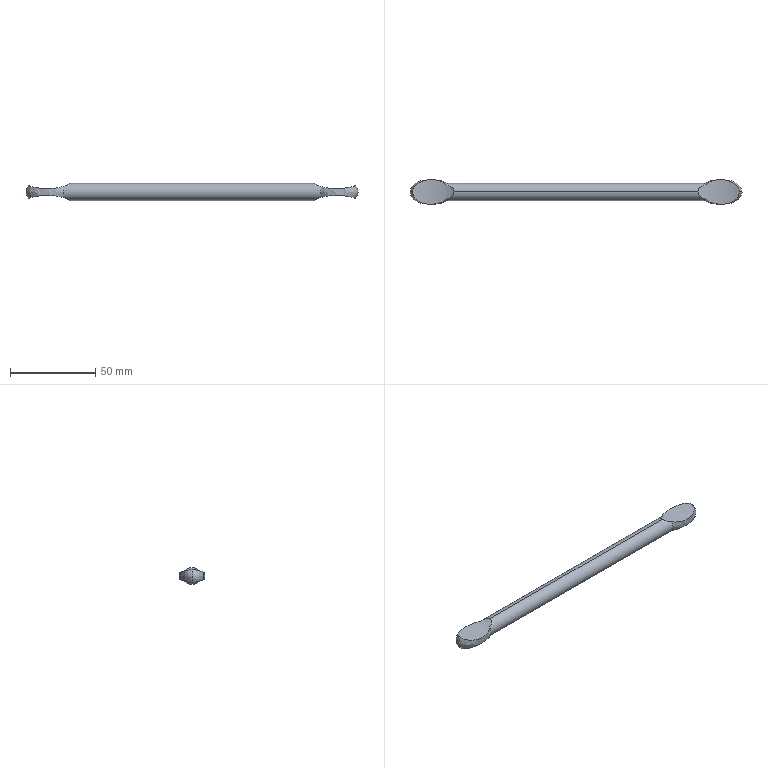Part | SolidWorks | features Extrusion 1, ICE 1, MirrorPattern 1, Revolution 1 | 1 solid | 10 faces | box 195 x 14.893 x 10 mm | volume 14339 mm3 | spline 8 | cylinder 2 | commonest cylinder face diameters 10 x2
STEP:
#1=CARTESIAN_POINT('',(97.5,0.,0.));
#2=VERTEX_POINT('',#1);
#3=CARTESIAN_POINT('',(95.865,0.,-3.708));
#4=VERTEX_POINT('',#3);
#5=CARTESIAN_POINT('',(97.5,0.,0.));
#6=CARTESIAN_POINT('',(97.5,0.,-1.308));
#7=CARTESIAN_POINT('',(96.943,0.,-2.572));
#8=CARTESIAN_POINT('',(95.865,0.,-3.708));
#9=(BOUNDED_CURVE()B_SPLINE_CURVE(3,(#5,#6,#7,#8),.UNSPECIFIED.,.F.,.T.)B_SPLINE_CURVE_WITH_KNOTS((4,4),(0.,0.5172),.UNSPECIFIED.)CURVE()GEOMETRIC_REPRESENTATION_ITEM()RATIONAL_B_SPLINE_CURVE((1.,0.9778,0.9778,1.))REPRESENTATION_ITEM(''));
#10=EDGE_CURVE('',#2,#4,#9,.T.);
#11=ORIENTED_EDGE('',*,*,#10,.F.);
#12=CARTESIAN_POINT('',(95.865,0.,3.708));
#13=VERTEX_POINT('',#12);
#14=CARTESIAN_POINT('',(97.5,0.,0.));
#15=CARTESIAN_POINT('',(97.5,0.,1.308));
#16=CARTESIAN_POINT('',(96.943,0.,2.572));
#17=CARTESIAN_POINT('',(95.865,0.,3.708));
#18=(BOUNDED_CURVE()B_SPLINE_CURVE(3,(#14,#15,#16,#17),.UNSPECIFIED.,.F.,.T.)B_SPLINE_CURVE_WITH_KNOTS((4,4),(0.,0.5172),.UNSPECIFIED.)CURVE()GEOMETRIC_REPRESENTATION_ITEM()RATIONAL_B_SPLINE_CURVE((1.,0.9778,0.9778,1.))REPRESENTATION_ITEM(''));
#19=EDGE_CURVE('',#2,#13,#18,.T.);
#20=ORIENTED_EDGE('',*,*,#19,.T.);
#21=CARTESIAN_POINT('',(75.683,-3.851,3.19));
#22=VERTEX_POINT('',#21);
#23=CARTESIAN_POINT('',(95.865,0.,3.708));
#24=CARTESIAN_POINT('',(95.865,-0.2608,3.708));
#25=CARTESIAN_POINT('',(95.846,-0.5214,3.701));
#26=CARTESIAN_POINT('',(95.771,-1.032,3.672));
#27=CARTESIAN_POINT('',(95.716,-1.283,3.651));
#28=CARTESIAN_POINT('',(95.569,-1.778,3.597));
#29=CARTESIAN_POINT('',(95.477,-2.023,3.564));
#30=CARTESIAN_POINT('',(95.265,-2.49,3.489));
#31=CARTESIAN_POINT('',(95.144,-2.715,3.448));
#32=CARTESIAN_POINT('',(94.875,-3.149,3.359));
#33=CARTESIAN_POINT('',(94.725,-3.359,3.312));
#34=CARTESIAN_POINT('',(94.406,-3.757,3.215));
#35=CARTESIAN_POINT('',(94.236,-3.945,3.166));
#36=CARTESIAN_POINT('',(93.701,-4.481,3.017));
#37=CARTESIAN_POINT('',(93.306,-4.803,2.917));
#38=CARTESIAN_POINT('',(92.462,-5.379,2.725));
#39=CARTESIAN_POINT('',(92.021,-5.629,2.636));
#40=CARTESIAN_POINT('',(91.107,-6.069,2.473));
#41=CARTESIAN_POINT('',(90.635,-6.259,2.399));
#42=CARTESIAN_POINT('',(89.662,-6.587,2.269));
#43=CARTESIAN_POINT('',(89.163,-6.725,2.213));
#44=CARTESIAN_POINT('',(88.157,-6.948,2.12));
#45=CARTESIAN_POINT('',(87.647,-7.035,2.083));
#46=CARTESIAN_POINT('',(86.619,-7.162,2.029));
#47=CARTESIAN_POINT('',(86.103,-7.202,2.012));
#48=CARTESIAN_POINT('',(85.068,-7.236,1.997));
#49=CARTESIAN_POINT('',(84.548,-7.23,1.999));
#50=CARTESIAN_POINT('',(82.998,-7.145,2.036));
#51=CARTESIAN_POINT('',(81.968,-6.997,2.1));
#52=CARTESIAN_POINT('',(80.468,-6.625,2.254));
#53=CARTESIAN_POINT('',(79.973,-6.474,2.315));
#54=CARTESIAN_POINT('',(79.014,-6.12,2.453));
#55=CARTESIAN_POINT('',(78.55,-5.916,2.531));
#56=CARTESIAN_POINT('',(77.656,-5.448,2.701));
#57=CARTESIAN_POINT('',(77.227,-5.183,2.793));
#58=CARTESIAN_POINT('',(76.614,-4.726,2.939));
#59=CARTESIAN_POINT('',(76.415,-4.564,2.989));
#60=CARTESIAN_POINT('',(76.035,-4.221,3.089));
#61=CARTESIAN_POINT('',(75.854,-4.041,3.14));
#62=CARTESIAN_POINT('',(75.683,-3.851,3.19));
#63=B_SPLINE_CURVE_WITH_KNOTS('',3,(#23,#24,#25,#26,#27,#28,#29,#30,#31,#32,#33,#34,#35,#36,#37,#38,#39,#40,#41,#42,#43,#44,#45,#46,#47,#48,#49,#50,#51,#52,#53,#54,#55,#56,#57,#58,#59,#60,#61,#62),.UNSPECIFIED.,.F.,.F.,(4,2,2,2,2,2,2,2,2,2,2,2,2,2,2,2,2,2,2,4),(0.02466,0.02543,0.0262,0.02697,0.02773,0.0285,0.02927,0.03081,0.03235,0.03389,0.03542,0.03696,0.0385,0.04004,0.04311,0.04465,0.04619,0.04773,0.04849,0.04926),.UNSPECIFIED.);
#64=EDGE_CURVE('',#13,#22,#63,.T.);
#65=ORIENTED_EDGE('',*,*,#64,.T.);
#66=CARTESIAN_POINT('',(75.683,-3.851,-3.19));
#67=VERTEX_POINT('',#66);
#68=CARTESIAN_POINT('',(75.683,0.,0.));
#69=DIRECTION('',(1.,0.,0.));
#70=DIRECTION('',(0.,0.,1.));
#71=AXIS2_PLACEMENT_3D('',#68,#69,#70);
#72=CIRCLE('',#71,5.);
#73=EDGE_CURVE('',#22,#67,#72,.T.);
#74=ORIENTED_EDGE('',*,*,#73,.T.);
#75=CARTESIAN_POINT('',(75.683,-3.851,-3.19));
#76=CARTESIAN_POINT('',(76.026,-4.232,-3.09));
#77=CARTESIAN_POINT('',(76.404,-4.569,-2.989));
#78=CARTESIAN_POINT('',(77.218,-5.177,-2.795));
#79=CARTESIAN_POINT('',(77.657,-5.448,-2.7));
#80=CARTESIAN_POINT('',(79.01,-6.157,-2.444));
#81=CARTESIAN_POINT('',(79.969,-6.501,-2.305));
#82=CARTESIAN_POINT('',(81.473,-6.874,-2.151));
#83=CARTESIAN_POINT('',(81.981,-6.973,-2.109));
#84=CARTESIAN_POINT('',(83.003,-7.123,-2.046));
#85=CARTESIAN_POINT('',(83.52,-7.174,-2.024));
#86=CARTESIAN_POINT('',(84.555,-7.23,-1.999));
#87=CARTESIAN_POINT('',(85.073,-7.236,-1.997));
#88=CARTESIAN_POINT('',(86.109,-7.201,-2.012));
#89=CARTESIAN_POINT('',(86.627,-7.161,-2.029));
#90=CARTESIAN_POINT('',(87.654,-7.034,-2.083));
#91=CARTESIAN_POINT('',(88.163,-6.947,-2.12));
#92=CARTESIAN_POINT('',(89.173,-6.722,-2.214));
#93=CARTESIAN_POINT('',(89.667,-6.586,-2.27));
#94=CARTESIAN_POINT('',(90.632,-6.26,-2.399));
#95=CARTESIAN_POINT('',(91.102,-6.072,-2.472));
#96=CARTESIAN_POINT('',(92.014,-5.633,-2.635));
#97=CARTESIAN_POINT('',(92.458,-5.381,-2.725));
#98=CARTESIAN_POINT('',(93.305,-4.804,-2.916));
#99=CARTESIAN_POINT('',(93.698,-4.483,-3.016));
#100=CARTESIAN_POINT('',(94.417,-3.765,-3.216));
#101=CARTESIAN_POINT('',(94.743,-3.362,-3.316));
#102=CARTESIAN_POINT('',(95.146,-2.712,-3.448));
#103=CARTESIAN_POINT('',(95.267,-2.487,-3.49));
#104=CARTESIAN_POINT('',(95.479,-2.019,-3.564));
#105=CARTESIAN_POINT('',(95.571,-1.774,-3.598));
#106=CARTESIAN_POINT('',(95.79,-1.032,-3.678));
#107=CARTESIAN_POINT('',(95.865,-0.5232,-3.708));
#108=CARTESIAN_POINT('',(95.865,0.,-3.708));
#109=B_SPLINE_CURVE_WITH_KNOTS('',3,(#75,#76,#77,#78,#79,#80,#81,#82,#83,#84,#85,#86,#87,#88,#89,#90,#91,#92,#93,#94,#95,#96,#97,#98,#99,#100,#101,#102,#103,#104,#105,#106,#107,#108),.UNSPECIFIED.,.F.,.F.,(4,2,2,2,2,2,2,2,2,2,2,2,2,2,2,2,4),(0.,0.00155,0.0031,0.0062,0.007749,0.009299,0.01085,0.0124,0.01395,0.0155,0.01705,0.0186,0.02015,0.0217,0.02247,0.02325,0.0248),.UNSPECIFIED.);
#110=EDGE_CURVE('',#67,#4,#109,.T.);
#111=ORIENTED_EDGE('',*,*,#110,.T.);
#112=EDGE_LOOP('',(#11,#20,#65,#74,#111));
#113=FACE_OUTER_BOUND('',#112,.T.);
#114=CARTESIAN_POINT('',(97.5,0.,0.));
#115=CARTESIAN_POINT('',(97.5,0.,0.));
#116=CARTESIAN_POINT('',(97.5,0.,0.));
#117=CARTESIAN_POINT('',(97.5,0.,0.));
#118=CARTESIAN_POINT('',(97.5,0.,-8.177));
#119=CARTESIAN_POINT('',(97.5,-16.354,-8.177));
#120=CARTESIAN_POINT('',(97.5,-16.354,8.177));
#121=CARTESIAN_POINT('',(97.5,0.,8.177));
#122=CARTESIAN_POINT('',(84.769,0.,-11.095));
#123=CARTESIAN_POINT('',(84.769,-22.19,-11.095));
#124=CARTESIAN_POINT('',(84.769,-22.19,11.095));
#125=CARTESIAN_POINT('',(84.769,0.,11.095));
#126=CARTESIAN_POINT('',(75.683,0.,-5.));
#127=CARTESIAN_POINT('',(75.683,-10.,-5.));
#128=CARTESIAN_POINT('',(75.683,-10.,5.));
#129=CARTESIAN_POINT('',(75.683,0.,5.));
#130=(BOUNDED_SURFACE()B_SPLINE_SURFACE(3,3,((#114,#115,#116,#117),(#118,#119,#120,#121),(#122,#123,#124,#125),(#126,#127,#128,#129)),.UNSPECIFIED.,.F.,.F.,.T.)B_SPLINE_SURFACE_WITH_KNOTS((4,4),(4,4),(0.,1.),(0.,1.),.UNSPECIFIED.)GEOMETRIC_REPRESENTATION_ITEM()RATIONAL_B_SPLINE_SURFACE(((1.,0.3333,0.3333,1.),(0.5712,0.1904,0.1904,0.5712),(0.5712,0.1904,0.1904,0.5712),(1.,0.3333,0.3333,1.)))REPRESENTATION_ITEM('')SURFACE());
#131=ADVANCED_FACE('',(#113),#130,.F.);
#132=CARTESIAN_POINT('',(-97.5,0.,0.));
#133=VERTEX_POINT('',#132);
#134=CARTESIAN_POINT('',(-95.865,0.,-3.708));
#135=VERTEX_POINT('',#134);
#136=CARTESIAN_POINT('',(-97.5,0.,0.));
#137=CARTESIAN_POINT('',(-97.5,0.,-1.308));
#138=CARTESIAN_POINT('',(-96.943,0.,-2.572));
#139=CARTESIAN_POINT('',(-95.865,0.,-3.708));
#140=(BOUNDED_CURVE()B_SPLINE_CURVE(3,(#136,#137,#138,#139),.UNSPECIFIED.,.F.,.T.)B_SPLINE_CURVE_WITH_KNOTS((4,4),(0.,0.5172),.UNSPECIFIED.)CURVE()GEOMETRIC_REPRESENTATION_ITEM()RATIONAL_B_SPLINE_CURVE((1.,0.9778,0.9778,1.))REPRESENTATION_ITEM(''));
#141=EDGE_CURVE('',#133,#135,#140,.T.);
#142=ORIENTED_EDGE('',*,*,#141,.F.);
#143=CARTESIAN_POINT('',(-95.865,0.,3.708));
#144=VERTEX_POINT('',#143);
#145=CARTESIAN_POINT('',(-97.5,0.,0.));
#146=CARTESIAN_POINT('',(-97.5,0.,1.308));
#147=CARTESIAN_POINT('',(-96.943,0.,2.572));
#148=CARTESIAN_POINT('',(-95.865,0.,3.708));
#149=(BOUNDED_CURVE()B_SPLINE_CURVE(3,(#145,#146,#147,#148),.UNSPECIFIED.,.F.,.T.)B_SPLINE_CURVE_WITH_KNOTS((4,4),(0.,0.5172),.UNSPECIFIED.)CURVE()GEOMETRIC_REPRESENTATION_ITEM()RATIONAL_B_SPLINE_CURVE((1.,0.9778,0.9778,1.))REPRESENTATION_ITEM(''));
#150=EDGE_CURVE('',#133,#144,#149,.T.);
#151=ORIENTED_EDGE('',*,*,#150,.T.);
#152=CARTESIAN_POINT('',(-75.683,3.851,3.19));
#153=VERTEX_POINT('',#152);
#154=CARTESIAN_POINT('',(-75.683,3.851,3.19));
#155=CARTESIAN_POINT('',(-76.025,4.231,3.09));
#156=CARTESIAN_POINT('',(-76.402,4.567,2.99));
#157=CARTESIAN_POINT('',(-77.21,5.172,2.796));
#158=CARTESIAN_POINT('',(-77.644,5.441,2.703));
#159=CARTESIAN_POINT('',(-79.003,6.154,2.445));
#160=CARTESIAN_POINT('',(-79.976,6.503,2.304));
#161=CARTESIAN_POINT('',(-81.978,6.999,2.099));
#162=CARTESIAN_POINT('',(-83.01,7.146,2.035));
#163=CARTESIAN_POINT('',(-84.562,7.231,1.999));
#164=CARTESIAN_POINT('',(-85.079,7.236,1.997));
#165=CARTESIAN_POINT('',(-86.114,7.201,2.012));
#166=CARTESIAN_POINT('',(-86.633,7.16,2.029));
#167=CARTESIAN_POINT('',(-87.659,7.033,2.084));
#168=CARTESIAN_POINT('',(-88.168,6.946,2.121));
#169=CARTESIAN_POINT('',(-89.177,6.721,2.214));
#170=CARTESIAN_POINT('',(-89.671,6.584,2.27));
#171=CARTESIAN_POINT('',(-90.635,6.259,2.399));
#172=CARTESIAN_POINT('',(-91.105,6.07,2.473));
#173=CARTESIAN_POINT('',(-92.017,5.631,2.635));
#174=CARTESIAN_POINT('',(-92.46,5.38,2.725));
#175=CARTESIAN_POINT('',(-93.306,4.802,2.917));
#176=CARTESIAN_POINT('',(-93.7,4.482,3.017));
#177=CARTESIAN_POINT('',(-94.418,3.763,3.216));
#178=CARTESIAN_POINT('',(-94.744,3.361,3.316));
#179=CARTESIAN_POINT('',(-95.146,2.711,3.449));
#180=CARTESIAN_POINT('',(-95.267,2.486,3.49));
#181=CARTESIAN_POINT('',(-95.479,2.018,3.564));
#182=CARTESIAN_POINT('',(-95.571,1.773,3.598));
#183=CARTESIAN_POINT('',(-95.79,1.031,3.679));
#184=CARTESIAN_POINT('',(-95.865,0.5228,3.708));
#185=CARTESIAN_POINT('',(-95.865,0.,3.708));
#186=B_SPLINE_CURVE_WITH_KNOTS('',3,(#154,#155,#156,#157,#158,#159,#160,#161,#162,#163,#164,#165,#166,#167,#168,#169,#170,#171,#172,#173,#174,#175,#176,#177,#178,#179,#180,#181,#182,#183,#184,#185),.UNSPECIFIED.,.F.,.F.,(4,2,2,2,2,2,2,2,2,2,2,2,2,2,2,4),(0.,0.001541,0.003082,0.006165,0.009247,0.01079,0.01233,0.01387,0.01541,0.01695,0.01849,0.02004,0.02158,0.02235,0.02312,0.02466),.UNSPECIFIED.);
#187=EDGE_CURVE('',#153,#144,#186,.T.);
#188=ORIENTED_EDGE('',*,*,#187,.F.);
#189=CARTESIAN_POINT('',(-75.683,3.851,-3.19));
#190=VERTEX_POINT('',#189);
#191=CARTESIAN_POINT('',(-75.683,0.,0.));
#192=DIRECTION('',(-1.,0.,0.));
#193=DIRECTION('',(0.,0.,-1.));
#194=AXIS2_PLACEMENT_3D('',#191,#192,#193);
#195=CIRCLE('',#194,5.);
#196=EDGE_CURVE('',#153,#190,#195,.T.);
#197=ORIENTED_EDGE('',*,*,#196,.T.);
#198=CARTESIAN_POINT('',(-95.865,0.,-3.708));
#199=CARTESIAN_POINT('',(-95.865,0.2609,-3.708));
#200=CARTESIAN_POINT('',(-95.846,0.5213,-3.701));
#201=CARTESIAN_POINT('',(-95.771,1.032,-3.672));
#202=CARTESIAN_POINT('',(-95.716,1.283,-3.651));
#203=CARTESIAN_POINT('',(-95.569,1.778,-3.597));
#204=CARTESIAN_POINT('',(-95.477,2.023,-3.564));
#205=CARTESIAN_POINT('',(-95.265,2.49,-3.489));
#206=CARTESIAN_POINT('',(-95.144,2.715,-3.448));
#207=CARTESIAN_POINT('',(-94.875,3.149,-3.359));
#208=CARTESIAN_POINT('',(-94.725,3.359,-3.312));
#209=CARTESIAN_POINT('',(-94.406,3.757,-3.215));
#210=CARTESIAN_POINT('',(-94.236,3.945,-3.166));
#211=CARTESIAN_POINT('',(-93.701,4.481,-3.017));
#212=CARTESIAN_POINT('',(-93.306,4.803,-2.917));
#213=CARTESIAN_POINT('',(-92.462,5.379,-2.725));
#214=CARTESIAN_POINT('',(-92.021,5.629,-2.636));
#215=CARTESIAN_POINT('',(-91.107,6.069,-2.473));
#216=CARTESIAN_POINT('',(-90.635,6.259,-2.399));
#217=CARTESIAN_POINT('',(-89.662,6.587,-2.269));
#218=CARTESIAN_POINT('',(-89.163,6.725,-2.213));
#219=CARTESIAN_POINT('',(-88.157,6.948,-2.12));
#220=CARTESIAN_POINT('',(-87.647,7.035,-2.083));
#221=CARTESIAN_POINT('',(-86.619,7.162,-2.029));
#222=CARTESIAN_POINT('',(-86.103,7.202,-2.012));
#223=CARTESIAN_POINT('',(-85.068,7.236,-1.997));
#224=CARTESIAN_POINT('',(-84.548,7.23,-1.999));
#225=CARTESIAN_POINT('',(-82.998,7.145,-2.036));
#226=CARTESIAN_POINT('',(-81.968,6.997,-2.1));
#227=CARTESIAN_POINT('',(-80.468,6.625,-2.254));
#228=CARTESIAN_POINT('',(-79.973,6.474,-2.315));
#229=CARTESIAN_POINT('',(-79.014,6.12,-2.453));
#230=CARTESIAN_POINT('',(-78.55,5.916,-2.531));
#231=CARTESIAN_POINT('',(-77.656,5.448,-2.701));
#232=CARTESIAN_POINT('',(-77.227,5.183,-2.793));
#233=CARTESIAN_POINT('',(-76.614,4.726,-2.939));
#234=CARTESIAN_POINT('',(-76.415,4.564,-2.989));
#235=CARTESIAN_POINT('',(-76.035,4.221,-3.089));
#236=CARTESIAN_POINT('',(-75.854,4.041,-3.14));
#237=CARTESIAN_POINT('',(-75.683,3.851,-3.19));
#238=B_SPLINE_CURVE_WITH_KNOTS('',3,(#198,#199,#200,#201,#202,#203,#204,#205,#206,#207,#208,#209,#210,#211,#212,#213,#214,#215,#216,#217,#218,#219,#220,#221,#222,#223,#224,#225,#226,#227,#228,#229,#230,#231,#232,#233,#234,#235,#236,#237),.UNSPECIFIED.,.F.,.F.,(4,2,2,2,2,2,2,2,2,2,2,2,2,2,2,2,2,2,2,4),(0.0248,0.02557,0.02634,0.02712,0.02789,0.02866,0.02944,0.03098,0.03253,0.03407,0.03562,0.03716,0.03871,0.04026,0.04335,0.04489,0.04644,0.04798,0.04876,0.04953),.UNSPECIFIED.);
#239=EDGE_CURVE('',#135,#190,#238,.T.);
#240=ORIENTED_EDGE('',*,*,#239,.F.);
#241=EDGE_LOOP('',(#142,#151,#188,#197,#240));
#242=FACE_OUTER_BOUND('',#241,.T.);
#243=CARTESIAN_POINT('',(-97.5,0.,0.));
#244=CARTESIAN_POINT('',(-97.5,0.,0.));
#245=CARTESIAN_POINT('',(-97.5,0.,0.));
#246=CARTESIAN_POINT('',(-97.5,0.,0.));
#247=CARTESIAN_POINT('',(-97.5,0.,-8.177));
#248=CARTESIAN_POINT('',(-97.5,16.354,-8.177));
#249=CARTESIAN_POINT('',(-97.5,16.354,8.177));
#250=CARTESIAN_POINT('',(-97.5,0.,8.177));
#251=CARTESIAN_POINT('',(-84.769,0.,-11.095));
#252=CARTESIAN_POINT('',(-84.769,22.19,-11.095));
#253=CARTESIAN_POINT('',(-84.769,22.19,11.095));
#254=CARTESIAN_POINT('',(-84.769,0.,11.095));
#255=CARTESIAN_POINT('',(-75.683,0.,-5.));
#256=CARTESIAN_POINT('',(-75.683,10.,-5.));
#257=CARTESIAN_POINT('',(-75.683,10.,5.));
#258=CARTESIAN_POINT('',(-75.683,0.,5.));
#259=(BOUNDED_SURFACE()B_SPLINE_SURFACE(3,3,((#243,#244,#245,#246),(#247,#248,#249,#250),(#251,#252,#253,#254),(#255,#256,#257,#258)),.UNSPECIFIED.,.F.,.F.,.T.)B_SPLINE_SURFACE_WITH_KNOTS((4,4),(4,4),(0.,1.),(0.,1.),.UNSPECIFIED.)GEOMETRIC_REPRESENTATION_ITEM()RATIONAL_B_SPLINE_SURFACE(((1.,0.3333,0.3333,1.),(0.5712,0.1904,0.1904,0.5712),(0.5712,0.1904,0.1904,0.5712),(1.,0.3333,0.3333,1.)))REPRESENTATION_ITEM('')SURFACE());
#260=ADVANCED_FACE('',(#242),#259,.F.);
#261=CARTESIAN_POINT('',(75.683,3.851,-3.19));
#262=VERTEX_POINT('',#261);
#263=CARTESIAN_POINT('',(71.639,0.,-5.));
#264=VERTEX_POINT('',#263);
#265=CARTESIAN_POINT('',(75.683,3.851,-3.19));
#266=CARTESIAN_POINT('',(75.185,3.731,-3.334));
#267=CARTESIAN_POINT('',(74.701,3.586,-3.494));
#268=CARTESIAN_POINT('',(74.008,3.303,-3.756));
#269=CARTESIAN_POINT('',(73.783,3.198,-3.847));
#270=CARTESIAN_POINT('',(73.346,2.956,-4.035));
#271=CARTESIAN_POINT('',(73.136,2.821,-4.132));
#272=CARTESIAN_POINT('',(72.747,2.515,-4.325));
#273=CARTESIAN_POINT('',(72.564,2.342,-4.423));
#274=CARTESIAN_POINT('',(72.242,1.959,-4.605));
#275=CARTESIAN_POINT('',(72.104,1.75,-4.69));
#276=CARTESIAN_POINT('',(71.875,1.294,-4.836));
#277=CARTESIAN_POINT('',(71.786,1.044,-4.897));
#278=CARTESIAN_POINT('',(71.699,0.6618,-4.958));
#279=CARTESIAN_POINT('',(71.676,0.5323,-4.973));
#280=CARTESIAN_POINT('',(71.647,0.2688,-4.995));
#281=CARTESIAN_POINT('',(71.639,0.1337,-5.));
#282=CARTESIAN_POINT('',(71.639,0.,-5.));
#283=B_SPLINE_CURVE_WITH_KNOTS('',3,(#265,#266,#267,#268,#269,#270,#271,#272,#273,#274,#275,#276,#277,#278,#279,#280,#281,#282),.UNSPECIFIED.,.F.,.F.,(4,2,2,2,2,2,2,2,4),(0.,0.001585,0.002377,0.00317,0.003962,0.004755,0.005547,0.005943,0.00634),.UNSPECIFIED.);
#284=EDGE_CURVE('',#262,#264,#283,.T.);
#285=ORIENTED_EDGE('',*,*,#284,.T.);
#286=CARTESIAN_POINT('',(-71.639,0.,-5.));
#287=VERTEX_POINT('',#286);
#288=CARTESIAN_POINT('',(85.,0.,-5.));
#289=DIRECTION('',(-1.,0.,0.));
#290=VECTOR('',#289,1000.);
#291=LINE('',#288,#290);
#292=EDGE_CURVE('',#264,#287,#291,.T.);
#293=ORIENTED_EDGE('',*,*,#292,.T.);
#294=CARTESIAN_POINT('',(-75.683,3.851,-3.19));
#295=CARTESIAN_POINT('',(-75.185,3.731,-3.334));
#296=CARTESIAN_POINT('',(-74.701,3.586,-3.494));
#297=CARTESIAN_POINT('',(-74.008,3.303,-3.756));
#298=CARTESIAN_POINT('',(-73.783,3.198,-3.847));
#299=CARTESIAN_POINT('',(-73.346,2.956,-4.035));
#300=CARTESIAN_POINT('',(-73.136,2.821,-4.132));
#301=CARTESIAN_POINT('',(-72.747,2.515,-4.325));
#302=CARTESIAN_POINT('',(-72.564,2.342,-4.423));
#303=CARTESIAN_POINT('',(-72.242,1.959,-4.605));
#304=CARTESIAN_POINT('',(-72.104,1.75,-4.69));
#305=CARTESIAN_POINT('',(-71.875,1.294,-4.836));
#306=CARTESIAN_POINT('',(-71.786,1.044,-4.897));
#307=CARTESIAN_POINT('',(-71.699,0.6618,-4.958));
#308=CARTESIAN_POINT('',(-71.676,0.5323,-4.973));
#309=CARTESIAN_POINT('',(-71.647,0.2688,-4.995));
#310=CARTESIAN_POINT('',(-71.639,0.1337,-5.));
#311=CARTESIAN_POINT('',(-71.639,0.,-5.));
#312=B_SPLINE_CURVE_WITH_KNOTS('',3,(#294,#295,#296,#297,#298,#299,#300,#301,#302,#303,#304,#305,#306,#307,#308,#309,#310,#311),.UNSPECIFIED.,.F.,.F.,(4,2,2,2,2,2,2,2,4),(0.,0.001585,0.002377,0.00317,0.003962,0.004755,0.005547,0.005943,0.00634),.UNSPECIFIED.);
#313=EDGE_CURVE('',#190,#287,#312,.T.);
#314=ORIENTED_EDGE('',*,*,#313,.F.);
#315=ORIENTED_EDGE('',*,*,#196,.F.);
#316=CARTESIAN_POINT('',(-71.639,0.,5.));
#317=VERTEX_POINT('',#316);
#318=CARTESIAN_POINT('',(-71.639,0.,5.));
#319=CARTESIAN_POINT('',(-71.639,0.2676,5.));
#320=CARTESIAN_POINT('',(-71.668,0.5298,4.979));
#321=CARTESIAN_POINT('',(-71.757,0.9154,4.917));
#322=CARTESIAN_POINT('',(-71.794,1.042,4.892));
#323=CARTESIAN_POINT('',(-71.881,1.287,4.833));
#324=CARTESIAN_POINT('',(-71.931,1.405,4.8));
#325=CARTESIAN_POINT('',(-72.102,1.747,4.691));
#326=CARTESIAN_POINT('',(-72.244,1.961,4.604));
#327=CARTESIAN_POINT('',(-72.565,2.343,4.422));
#328=CARTESIAN_POINT('',(-72.747,2.515,4.325));
#329=CARTESIAN_POINT('',(-73.331,2.974,4.036));
#330=CARTESIAN_POINT('',(-73.768,3.205,3.846));
#331=CARTESIAN_POINT('',(-74.7,3.586,3.494));
#332=CARTESIAN_POINT('',(-75.185,3.731,3.334));
#333=CARTESIAN_POINT('',(-75.683,3.851,3.19));
#334=B_SPLINE_CURVE_WITH_KNOTS('',3,(#318,#319,#320,#321,#322,#323,#324,#325,#326,#327,#328,#329,#330,#331,#332,#333),.UNSPECIFIED.,.F.,.F.,(4,2,2,2,2,2,2,4),(0.006337,0.007126,0.007521,0.007915,0.008704,0.009494,0.01107,0.01265),.UNSPECIFIED.);
#335=EDGE_CURVE('',#317,#153,#334,.T.);
#336=ORIENTED_EDGE('',*,*,#335,.F.);
#337=CARTESIAN_POINT('',(71.639,0.,5.));
#338=VERTEX_POINT('',#337);
#339=CARTESIAN_POINT('',(85.,0.,5.));
#340=DIRECTION('',(-1.,0.,0.));
#341=VECTOR('',#340,1000.);
#342=LINE('',#339,#341);
#343=EDGE_CURVE('',#338,#317,#342,.T.);
#344=ORIENTED_EDGE('',*,*,#343,.F.);
#345=CARTESIAN_POINT('',(75.683,3.851,3.19));
#346=VERTEX_POINT('',#345);
#347=CARTESIAN_POINT('',(71.639,0.,5.));
#348=CARTESIAN_POINT('',(71.639,0.2676,5.));
#349=CARTESIAN_POINT('',(71.668,0.5298,4.979));
#350=CARTESIAN_POINT('',(71.757,0.9154,4.917));
#351=CARTESIAN_POINT('',(71.794,1.042,4.892));
#352=CARTESIAN_POINT('',(71.881,1.287,4.833));
#353=CARTESIAN_POINT('',(71.931,1.405,4.8));
#354=CARTESIAN_POINT('',(72.102,1.747,4.691));
#355=CARTESIAN_POINT('',(72.244,1.961,4.604));
#356=CARTESIAN_POINT('',(72.565,2.343,4.422));
#357=CARTESIAN_POINT('',(72.747,2.515,4.325));
#358=CARTESIAN_POINT('',(73.331,2.974,4.036));
#359=CARTESIAN_POINT('',(73.768,3.205,3.846));
#360=CARTESIAN_POINT('',(74.7,3.586,3.494));
#361=CARTESIAN_POINT('',(75.185,3.731,3.334));
#362=CARTESIAN_POINT('',(75.683,3.851,3.19));
#363=B_SPLINE_CURVE_WITH_KNOTS('',3,(#347,#348,#349,#350,#351,#352,#353,#354,#355,#356,#357,#358,#359,#360,#361,#362),.UNSPECIFIED.,.F.,.F.,(4,2,2,2,2,2,2,4),(0.006337,0.007126,0.007521,0.007915,0.008704,0.009494,0.01107,0.01265),.UNSPECIFIED.);
#364=EDGE_CURVE('',#338,#346,#363,.T.);
#365=ORIENTED_EDGE('',*,*,#364,.T.);
#366=CARTESIAN_POINT('',(75.683,0.,0.));
#367=DIRECTION('',(1.,0.,0.));
#368=DIRECTION('',(0.,0.,1.));
#369=AXIS2_PLACEMENT_3D('',#366,#367,#368);
#370=CIRCLE('',#369,5.);
#371=EDGE_CURVE('',#262,#346,#370,.T.);
#372=ORIENTED_EDGE('',*,*,#371,.F.);
#373=EDGE_LOOP('',(#285,#293,#314,#315,#336,#344,#365,#372));
#374=FACE_OUTER_BOUND('',#373,.T.);
#375=CARTESIAN_POINT('',(85.,0.,0.));
#376=DIRECTION('',(-1.,0.,0.));
#377=DIRECTION('',(0.,0.,1.));
#378=AXIS2_PLACEMENT_3D('',#375,#376,#377);
#379=CYLINDRICAL_SURFACE('',#378,5.);
#380=ADVANCED_FACE('',(#374),#379,.T.);
#381=ORIENTED_EDGE('',*,*,#292,.F.);
#382=CARTESIAN_POINT('',(71.639,0.,-5.));
#383=CARTESIAN_POINT('',(71.639,-0.2666,-5.));
#384=CARTESIAN_POINT('',(71.668,-0.5289,-4.979));
#385=CARTESIAN_POINT('',(71.786,-1.045,-4.897));
#386=CARTESIAN_POINT('',(71.874,-1.29,-4.837));
#387=CARTESIAN_POINT('',(72.102,-1.748,-4.691));
#388=CARTESIAN_POINT('',(72.244,-1.961,-4.604));
#389=CARTESIAN_POINT('',(72.565,-2.342,-4.422));
#390=CARTESIAN_POINT('',(72.747,-2.515,-4.325));
#391=CARTESIAN_POINT('',(73.136,-2.821,-4.132));
#392=CARTESIAN_POINT('',(73.343,-2.954,-4.037));
#393=CARTESIAN_POINT('',(73.775,-3.194,-3.85));
#394=CARTESIAN_POINT('',(74.002,-3.301,-3.758));
#395=CARTESIAN_POINT('',(74.7,-3.586,-3.494));
#396=CARTESIAN_POINT('',(75.185,-3.731,-3.334));
#397=CARTESIAN_POINT('',(75.683,-3.851,-3.19));
#398=B_SPLINE_CURVE_WITH_KNOTS('',3,(#382,#383,#384,#385,#386,#387,#388,#389,#390,#391,#392,#393,#394,#395,#396,#397),.UNSPECIFIED.,.F.,.F.,(4,2,2,2,2,2,2,4),(0.00634,0.00713,0.00792,0.00871,0.0095,0.01029,0.01108,0.01266),.UNSPECIFIED.);
#399=EDGE_CURVE('',#264,#67,#398,.T.);
#400=ORIENTED_EDGE('',*,*,#399,.T.);
#401=ORIENTED_EDGE('',*,*,#73,.F.);
#402=CARTESIAN_POINT('',(75.683,-3.851,3.19));
#403=CARTESIAN_POINT('',(75.185,-3.731,3.334));
#404=CARTESIAN_POINT('',(74.701,-3.586,3.494));
#405=CARTESIAN_POINT('',(74.008,-3.304,3.755));
#406=CARTESIAN_POINT('',(73.783,-3.198,3.846));
#407=CARTESIAN_POINT('',(73.347,-2.957,4.035));
#408=CARTESIAN_POINT('',(73.136,-2.821,4.132));
#409=CARTESIAN_POINT('',(72.747,-2.515,4.325));
#410=CARTESIAN_POINT('',(72.565,-2.343,4.422));
#411=CARTESIAN_POINT('',(72.242,-1.958,4.605));
#412=CARTESIAN_POINT('',(72.104,-1.75,4.69));
#413=CARTESIAN_POINT('',(71.876,-1.295,4.835));
#414=CARTESIAN_POINT('',(71.786,-1.044,4.897));
#415=CARTESIAN_POINT('',(71.669,-0.5335,4.978));
#416=CARTESIAN_POINT('',(71.639,-0.2686,5.));
#417=CARTESIAN_POINT('',(71.639,0.,5.));
#418=B_SPLINE_CURVE_WITH_KNOTS('',3,(#402,#403,#404,#405,#406,#407,#408,#409,#410,#411,#412,#413,#414,#415,#416,#417),.UNSPECIFIED.,.F.,.F.,(4,2,2,2,2,2,2,4),(0.,0.001584,0.002376,0.003169,0.003961,0.004753,0.005545,0.006337),.UNSPECIFIED.);
#419=EDGE_CURVE('',#22,#338,#418,.T.);
#420=ORIENTED_EDGE('',*,*,#419,.T.);
#421=ORIENTED_EDGE('',*,*,#343,.T.);
#422=CARTESIAN_POINT('',(-75.683,-3.851,3.19));
#423=VERTEX_POINT('',#422);
#424=CARTESIAN_POINT('',(-75.683,-3.851,3.19));
#425=CARTESIAN_POINT('',(-75.185,-3.731,3.334));
#426=CARTESIAN_POINT('',(-74.701,-3.586,3.494));
#427=CARTESIAN_POINT('',(-74.008,-3.304,3.755));
#428=CARTESIAN_POINT('',(-73.783,-3.198,3.846));
#429=CARTESIAN_POINT('',(-73.347,-2.957,4.035));
#430=CARTESIAN_POINT('',(-73.136,-2.821,4.132));
#431=CARTESIAN_POINT('',(-72.747,-2.515,4.325));
#432=CARTESIAN_POINT('',(-72.565,-2.343,4.422));
#433=CARTESIAN_POINT('',(-72.242,-1.958,4.605));
#434=CARTESIAN_POINT('',(-72.104,-1.75,4.69));
#435=CARTESIAN_POINT('',(-71.876,-1.295,4.835));
#436=CARTESIAN_POINT('',(-71.786,-1.044,4.897));
#437=CARTESIAN_POINT('',(-71.669,-0.5335,4.978));
#438=CARTESIAN_POINT('',(-71.639,-0.2686,5.));
#439=CARTESIAN_POINT('',(-71.639,0.,5.));
#440=B_SPLINE_CURVE_WITH_KNOTS('',3,(#424,#425,#426,#427,#428,#429,#430,#431,#432,#433,#434,#435,#436,#437,#438,#439),.UNSPECIFIED.,.F.,.F.,(4,2,2,2,2,2,2,4),(0.,0.001584,0.002376,0.003169,0.003961,0.004753,0.005545,0.006337),.UNSPECIFIED.);
#441=EDGE_CURVE('',#423,#317,#440,.T.);
#442=ORIENTED_EDGE('',*,*,#441,.F.);
#443=CARTESIAN_POINT('',(-75.683,-3.851,-3.19));
#444=VERTEX_POINT('',#443);
#445=CARTESIAN_POINT('',(-75.683,0.,0.));
#446=DIRECTION('',(-1.,0.,0.));
#447=DIRECTION('',(0.,0.,-1.));
#448=AXIS2_PLACEMENT_3D('',#445,#446,#447);
#449=CIRCLE('',#448,5.);
#450=EDGE_CURVE('',#444,#423,#449,.T.);
#451=ORIENTED_EDGE('',*,*,#450,.F.);
#452=CARTESIAN_POINT('',(-71.639,0.,-5.));
#453=CARTESIAN_POINT('',(-71.639,-0.2666,-5.));
#454=CARTESIAN_POINT('',(-71.668,-0.5289,-4.979));
#455=CARTESIAN_POINT('',(-71.786,-1.045,-4.897));
#456=CARTESIAN_POINT('',(-71.874,-1.29,-4.837));
#457=CARTESIAN_POINT('',(-72.102,-1.748,-4.691));
#458=CARTESIAN_POINT('',(-72.244,-1.961,-4.604));
#459=CARTESIAN_POINT('',(-72.565,-2.342,-4.422));
#460=CARTESIAN_POINT('',(-72.747,-2.515,-4.325));
#461=CARTESIAN_POINT('',(-73.136,-2.821,-4.132));
#462=CARTESIAN_POINT('',(-73.343,-2.954,-4.037));
#463=CARTESIAN_POINT('',(-73.775,-3.194,-3.85));
#464=CARTESIAN_POINT('',(-74.002,-3.301,-3.758));
#465=CARTESIAN_POINT('',(-74.7,-3.586,-3.494));
#466=CARTESIAN_POINT('',(-75.185,-3.731,-3.334));
#467=CARTESIAN_POINT('',(-75.683,-3.851,-3.19));
#468=B_SPLINE_CURVE_WITH_KNOTS('',3,(#452,#453,#454,#455,#456,#457,#458,#459,#460,#461,#462,#463,#464,#465,#466,#467),.UNSPECIFIED.,.F.,.F.,(4,2,2,2,2,2,2,4),(0.00634,0.00713,0.00792,0.00871,0.0095,0.01029,0.01108,0.01266),.UNSPECIFIED.);
#469=EDGE_CURVE('',#287,#444,#468,.T.);
#470=ORIENTED_EDGE('',*,*,#469,.F.);
#471=EDGE_LOOP('',(#381,#400,#401,#420,#421,#442,#451,#470));
#472=FACE_OUTER_BOUND('',#471,.T.);
#473=CARTESIAN_POINT('',(85.,0.,0.));
#474=DIRECTION('',(-1.,0.,0.));
#475=DIRECTION('',(0.,0.,1.));
#476=AXIS2_PLACEMENT_3D('',#473,#474,#475);
#477=CYLINDRICAL_SURFACE('',#476,5.);
#478=ADVANCED_FACE('',(#472),#477,.T.);
#479=ORIENTED_EDGE('',*,*,#150,.F.);
#480=ORIENTED_EDGE('',*,*,#141,.T.);
#481=CARTESIAN_POINT('',(-75.683,-3.851,-3.19));
#482=CARTESIAN_POINT('',(-76.026,-4.232,-3.09));
#483=CARTESIAN_POINT('',(-76.404,-4.569,-2.989));
#484=CARTESIAN_POINT('',(-77.218,-5.177,-2.795));
#485=CARTESIAN_POINT('',(-77.657,-5.448,-2.7));
#486=CARTESIAN_POINT('',(-79.01,-6.157,-2.444));
#487=CARTESIAN_POINT('',(-79.969,-6.501,-2.305));
#488=CARTESIAN_POINT('',(-81.473,-6.874,-2.151));
#489=CARTESIAN_POINT('',(-81.981,-6.973,-2.109));
#490=CARTESIAN_POINT('',(-83.003,-7.123,-2.046));
#491=CARTESIAN_POINT('',(-83.52,-7.174,-2.024));
#492=CARTESIAN_POINT('',(-84.555,-7.23,-1.999));
#493=CARTESIAN_POINT('',(-85.073,-7.236,-1.997));
#494=CARTESIAN_POINT('',(-86.109,-7.201,-2.012));
#495=CARTESIAN_POINT('',(-86.627,-7.161,-2.029));
#496=CARTESIAN_POINT('',(-87.654,-7.034,-2.083));
#497=CARTESIAN_POINT('',(-88.163,-6.947,-2.12));
#498=CARTESIAN_POINT('',(-89.173,-6.722,-2.214));
#499=CARTESIAN_POINT('',(-89.667,-6.586,-2.27));
#500=CARTESIAN_POINT('',(-90.632,-6.26,-2.399));
#501=CARTESIAN_POINT('',(-91.102,-6.072,-2.472));
#502=CARTESIAN_POINT('',(-92.014,-5.633,-2.635));
#503=CARTESIAN_POINT('',(-92.458,-5.381,-2.725));
#504=CARTESIAN_POINT('',(-93.305,-4.804,-2.916));
#505=CARTESIAN_POINT('',(-93.698,-4.483,-3.016));
#506=CARTESIAN_POINT('',(-94.417,-3.765,-3.216));
#507=CARTESIAN_POINT('',(-94.743,-3.362,-3.316));
#508=CARTESIAN_POINT('',(-95.146,-2.712,-3.448));
#509=CARTESIAN_POINT('',(-95.267,-2.487,-3.49));
#510=CARTESIAN_POINT('',(-95.479,-2.019,-3.564));
#511=CARTESIAN_POINT('',(-95.571,-1.774,-3.598));
#512=CARTESIAN_POINT('',(-95.79,-1.032,-3.678));
#513=CARTESIAN_POINT('',(-95.865,-0.5232,-3.708));
#514=CARTESIAN_POINT('',(-95.865,0.,-3.708));
#515=B_SPLINE_CURVE_WITH_KNOTS('',3,(#481,#482,#483,#484,#485,#486,#487,#488,#489,#490,#491,#492,#493,#494,#495,#496,#497,#498,#499,#500,#501,#502,#503,#504,#505,#506,#507,#508,#509,#510,#511,#512,#513,#514),.UNSPECIFIED.,.F.,.F.,(4,2,2,2,2,2,2,2,2,2,2,2,2,2,2,2,4),(0.,0.00155,0.0031,0.0062,0.007749,0.009299,0.01085,0.0124,0.01395,0.0155,0.01705,0.0186,0.02015,0.0217,0.02247,0.02325,0.0248),.UNSPECIFIED.);
#516=EDGE_CURVE('',#444,#135,#515,.T.);
#517=ORIENTED_EDGE('',*,*,#516,.F.);
#518=ORIENTED_EDGE('',*,*,#450,.T.);
#519=CARTESIAN_POINT('',(-95.865,0.,3.708));
#520=CARTESIAN_POINT('',(-95.865,-0.2608,3.708));
#521=CARTESIAN_POINT('',(-95.846,-0.5214,3.701));
#522=CARTESIAN_POINT('',(-95.771,-1.032,3.672));
#523=CARTESIAN_POINT('',(-95.716,-1.283,3.651));
#524=CARTESIAN_POINT('',(-95.569,-1.778,3.597));
#525=CARTESIAN_POINT('',(-95.477,-2.023,3.564));
#526=CARTESIAN_POINT('',(-95.265,-2.49,3.489));
#527=CARTESIAN_POINT('',(-95.144,-2.715,3.448));
#528=CARTESIAN_POINT('',(-94.875,-3.149,3.359));
#529=CARTESIAN_POINT('',(-94.725,-3.359,3.312));
#530=CARTESIAN_POINT('',(-94.406,-3.757,3.215));
#531=CARTESIAN_POINT('',(-94.236,-3.945,3.166));
#532=CARTESIAN_POINT('',(-93.701,-4.481,3.017));
#533=CARTESIAN_POINT('',(-93.306,-4.803,2.917));
#534=CARTESIAN_POINT('',(-92.462,-5.379,2.725));
#535=CARTESIAN_POINT('',(-92.021,-5.629,2.636));
#536=CARTESIAN_POINT('',(-91.107,-6.069,2.473));
#537=CARTESIAN_POINT('',(-90.635,-6.259,2.399));
#538=CARTESIAN_POINT('',(-89.662,-6.587,2.269));
#539=CARTESIAN_POINT('',(-89.163,-6.725,2.213));
#540=CARTESIAN_POINT('',(-88.157,-6.948,2.12));
#541=CARTESIAN_POINT('',(-87.647,-7.035,2.083));
#542=CARTESIAN_POINT('',(-86.619,-7.162,2.029));
#543=CARTESIAN_POINT('',(-86.103,-7.202,2.012));
#544=CARTESIAN_POINT('',(-85.068,-7.236,1.997));
#545=CARTESIAN_POINT('',(-84.548,-7.23,1.999));
#546=CARTESIAN_POINT('',(-82.998,-7.145,2.036));
#547=CARTESIAN_POINT('',(-81.968,-6.997,2.1));
#548=CARTESIAN_POINT('',(-80.468,-6.625,2.254));
#549=CARTESIAN_POINT('',(-79.973,-6.474,2.315));
#550=CARTESIAN_POINT('',(-79.014,-6.12,2.453));
#551=CARTESIAN_POINT('',(-78.55,-5.916,2.531));
#552=CARTESIAN_POINT('',(-77.656,-5.448,2.701));
#553=CARTESIAN_POINT('',(-77.227,-5.183,2.793));
#554=CARTESIAN_POINT('',(-76.614,-4.726,2.939));
#555=CARTESIAN_POINT('',(-76.415,-4.564,2.989));
#556=CARTESIAN_POINT('',(-76.035,-4.221,3.089));
#557=CARTESIAN_POINT('',(-75.854,-4.041,3.14));
#558=CARTESIAN_POINT('',(-75.683,-3.851,3.19));
#559=B_SPLINE_CURVE_WITH_KNOTS('',3,(#519,#520,#521,#522,#523,#524,#525,#526,#527,#528,#529,#530,#531,#532,#533,#534,#535,#536,#537,#538,#539,#540,#541,#542,#543,#544,#545,#546,#547,#548,#549,#550,#551,#552,#553,#554,#555,#556,#557,#558),.UNSPECIFIED.,.F.,.F.,(4,2,2,2,2,2,2,2,2,2,2,2,2,2,2,2,2,2,2,4),(0.02466,0.02543,0.0262,0.02697,0.02773,0.0285,0.02927,0.03081,0.03235,0.03389,0.03542,0.03696,0.0385,0.04004,0.04311,0.04465,0.04619,0.04773,0.04849,0.04926),.UNSPECIFIED.);
#560=EDGE_CURVE('',#144,#423,#559,.T.);
#561=ORIENTED_EDGE('',*,*,#560,.F.);
#562=EDGE_LOOP('',(#479,#480,#517,#518,#561));
#563=FACE_OUTER_BOUND('',#562,.T.);
#564=CARTESIAN_POINT('',(-97.5,0.,0.));
#565=CARTESIAN_POINT('',(-97.5,0.,0.));
#566=CARTESIAN_POINT('',(-97.5,0.,0.));
#567=CARTESIAN_POINT('',(-97.5,0.,0.));
#568=CARTESIAN_POINT('',(-97.5,0.,8.177));
#569=CARTESIAN_POINT('',(-97.5,-16.354,8.177));
#570=CARTESIAN_POINT('',(-97.5,-16.354,-8.177));
#571=CARTESIAN_POINT('',(-97.5,0.,-8.177));
#572=CARTESIAN_POINT('',(-84.769,0.,11.095));
#573=CARTESIAN_POINT('',(-84.769,-22.19,11.095));
#574=CARTESIAN_POINT('',(-84.769,-22.19,-11.095));
#575=CARTESIAN_POINT('',(-84.769,0.,-11.095));
#576=CARTESIAN_POINT('',(-75.683,0.,5.));
#577=CARTESIAN_POINT('',(-75.683,-10.,5.));
#578=CARTESIAN_POINT('',(-75.683,-10.,-5.));
#579=CARTESIAN_POINT('',(-75.683,0.,-5.));
#580=(BOUNDED_SURFACE()B_SPLINE_SURFACE(3,3,((#564,#565,#566,#567),(#568,#569,#570,#571),(#572,#573,#574,#575),(#576,#577,#578,#579)),.UNSPECIFIED.,.F.,.F.,.T.)B_SPLINE_SURFACE_WITH_KNOTS((4,4),(4,4),(0.,1.),(0.,1.),.UNSPECIFIED.)GEOMETRIC_REPRESENTATION_ITEM()RATIONAL_B_SPLINE_SURFACE(((1.,0.3333,0.3333,1.),(0.5712,0.1904,0.1904,0.5712),(0.5712,0.1904,0.1904,0.5712),(1.,0.3333,0.3333,1.)))REPRESENTATION_ITEM('')SURFACE());
#581=ADVANCED_FACE('',(#563),#580,.F.);
#582=ORIENTED_EDGE('',*,*,#19,.F.);
#583=ORIENTED_EDGE('',*,*,#10,.T.);
#584=CARTESIAN_POINT('',(95.865,0.,-3.708));
#585=CARTESIAN_POINT('',(95.865,0.2609,-3.708));
#586=CARTESIAN_POINT('',(95.846,0.5213,-3.701));
#587=CARTESIAN_POINT('',(95.771,1.032,-3.672));
#588=CARTESIAN_POINT('',(95.716,1.283,-3.651));
#589=CARTESIAN_POINT('',(95.569,1.778,-3.597));
#590=CARTESIAN_POINT('',(95.477,2.023,-3.564));
#591=CARTESIAN_POINT('',(95.265,2.49,-3.489));
#592=CARTESIAN_POINT('',(95.144,2.715,-3.448));
#593=CARTESIAN_POINT('',(94.875,3.149,-3.359));
#594=CARTESIAN_POINT('',(94.725,3.359,-3.312));
#595=CARTESIAN_POINT('',(94.406,3.757,-3.215));
#596=CARTESIAN_POINT('',(94.236,3.945,-3.166));
#597=CARTESIAN_POINT('',(93.701,4.481,-3.017));
#598=CARTESIAN_POINT('',(93.306,4.803,-2.917));
#599=CARTESIAN_POINT('',(92.462,5.379,-2.725));
#600=CARTESIAN_POINT('',(92.021,5.629,-2.636));
#601=CARTESIAN_POINT('',(91.107,6.069,-2.473));
#602=CARTESIAN_POINT('',(90.635,6.259,-2.399));
#603=CARTESIAN_POINT('',(89.662,6.587,-2.269));
#604=CARTESIAN_POINT('',(89.163,6.725,-2.213));
#605=CARTESIAN_POINT('',(88.157,6.948,-2.12));
#606=CARTESIAN_POINT('',(87.647,7.035,-2.083));
#607=CARTESIAN_POINT('',(86.619,7.162,-2.029));
#608=CARTESIAN_POINT('',(86.103,7.202,-2.012));
#609=CARTESIAN_POINT('',(85.068,7.236,-1.997));
#610=CARTESIAN_POINT('',(84.548,7.23,-1.999));
#611=CARTESIAN_POINT('',(82.998,7.145,-2.036));
#612=CARTESIAN_POINT('',(81.968,6.997,-2.1));
#613=CARTESIAN_POINT('',(80.468,6.625,-2.254));
#614=CARTESIAN_POINT('',(79.973,6.474,-2.315));
#615=CARTESIAN_POINT('',(79.014,6.12,-2.453));
#616=CARTESIAN_POINT('',(78.55,5.916,-2.531));
#617=CARTESIAN_POINT('',(77.656,5.448,-2.701));
#618=CARTESIAN_POINT('',(77.227,5.183,-2.793));
#619=CARTESIAN_POINT('',(76.614,4.726,-2.939));
#620=CARTESIAN_POINT('',(76.415,4.564,-2.989));
#621=CARTESIAN_POINT('',(76.035,4.221,-3.089));
#622=CARTESIAN_POINT('',(75.854,4.041,-3.14));
#623=CARTESIAN_POINT('',(75.683,3.851,-3.19));
#624=B_SPLINE_CURVE_WITH_KNOTS('',3,(#584,#585,#586,#587,#588,#589,#590,#591,#592,#593,#594,#595,#596,#597,#598,#599,#600,#601,#602,#603,#604,#605,#606,#607,#608,#609,#610,#611,#612,#613,#614,#615,#616,#617,#618,#619,#620,#621,#622,#623),.UNSPECIFIED.,.F.,.F.,(4,2,2,2,2,2,2,2,2,2,2,2,2,2,2,2,2,2,2,4),(0.0248,0.02557,0.02634,0.02712,0.02789,0.02866,0.02944,0.03098,0.03253,0.03407,0.03562,0.03716,0.03871,0.04026,0.04335,0.04489,0.04644,0.04798,0.04876,0.04953),.UNSPECIFIED.);
#625=EDGE_CURVE('',#4,#262,#624,.T.);
#626=ORIENTED_EDGE('',*,*,#625,.T.);
#627=ORIENTED_EDGE('',*,*,#371,.T.);
#628=CARTESIAN_POINT('',(75.683,3.851,3.19));
#629=CARTESIAN_POINT('',(76.025,4.231,3.09));
#630=CARTESIAN_POINT('',(76.402,4.567,2.99));
#631=CARTESIAN_POINT('',(77.21,5.172,2.796));
#632=CARTESIAN_POINT('',(77.644,5.441,2.703));
#633=CARTESIAN_POINT('',(79.003,6.154,2.445));
#634=CARTESIAN_POINT('',(79.976,6.503,2.304));
#635=CARTESIAN_POINT('',(81.978,6.999,2.099));
#636=CARTESIAN_POINT('',(83.01,7.146,2.035));
#637=CARTESIAN_POINT('',(84.562,7.231,1.999));
#638=CARTESIAN_POINT('',(85.079,7.236,1.997));
#639=CARTESIAN_POINT('',(86.114,7.201,2.012));
#640=CARTESIAN_POINT('',(86.633,7.16,2.029));
#641=CARTESIAN_POINT('',(87.659,7.033,2.084));
#642=CARTESIAN_POINT('',(88.168,6.946,2.121));
#643=CARTESIAN_POINT('',(89.177,6.721,2.214));
#644=CARTESIAN_POINT('',(89.671,6.584,2.27));
#645=CARTESIAN_POINT('',(90.635,6.259,2.399));
#646=CARTESIAN_POINT('',(91.105,6.07,2.473));
#647=CARTESIAN_POINT('',(92.017,5.631,2.635));
#648=CARTESIAN_POINT('',(92.46,5.38,2.725));
#649=CARTESIAN_POINT('',(93.306,4.802,2.917));
#650=CARTESIAN_POINT('',(93.7,4.482,3.017));
#651=CARTESIAN_POINT('',(94.418,3.763,3.216));
#652=CARTESIAN_POINT('',(94.744,3.361,3.316));
#653=CARTESIAN_POINT('',(95.146,2.711,3.449));
#654=CARTESIAN_POINT('',(95.267,2.486,3.49));
#655=CARTESIAN_POINT('',(95.479,2.018,3.564));
#656=CARTESIAN_POINT('',(95.571,1.773,3.598));
#657=CARTESIAN_POINT('',(95.79,1.031,3.679));
#658=CARTESIAN_POINT('',(95.865,0.5228,3.708));
#659=CARTESIAN_POINT('',(95.865,0.,3.708));
#660=B_SPLINE_CURVE_WITH_KNOTS('',3,(#628,#629,#630,#631,#632,#633,#634,#635,#636,#637,#638,#639,#640,#641,#642,#643,#644,#645,#646,#647,#648,#649,#650,#651,#652,#653,#654,#655,#656,#657,#658,#659),.UNSPECIFIED.,.F.,.F.,(4,2,2,2,2,2,2,2,2,2,2,2,2,2,2,4),(0.,0.001541,0.003082,0.006165,0.009247,0.01079,0.01233,0.01387,0.01541,0.01695,0.01849,0.02004,0.02158,0.02235,0.02312,0.02466),.UNSPECIFIED.);
#661=EDGE_CURVE('',#346,#13,#660,.T.);
#662=ORIENTED_EDGE('',*,*,#661,.T.);
#663=EDGE_LOOP('',(#582,#583,#626,#627,#662));
#664=FACE_OUTER_BOUND('',#663,.T.);
#665=CARTESIAN_POINT('',(97.5,0.,0.));
#666=CARTESIAN_POINT('',(97.5,0.,0.));
#667=CARTESIAN_POINT('',(97.5,0.,0.));
#668=CARTESIAN_POINT('',(97.5,0.,0.));
#669=CARTESIAN_POINT('',(97.5,0.,8.177));
#670=CARTESIAN_POINT('',(97.5,16.354,8.177));
#671=CARTESIAN_POINT('',(97.5,16.354,-8.177));
#672=CARTESIAN_POINT('',(97.5,0.,-8.177));
#673=CARTESIAN_POINT('',(84.769,0.,11.095));
#674=CARTESIAN_POINT('',(84.769,22.19,11.095));
#675=CARTESIAN_POINT('',(84.769,22.19,-11.095));
#676=CARTESIAN_POINT('',(84.769,0.,-11.095));
#677=CARTESIAN_POINT('',(75.683,0.,5.));
#678=CARTESIAN_POINT('',(75.683,10.,5.));
#679=CARTESIAN_POINT('',(75.683,10.,-5.));
#680=CARTESIAN_POINT('',(75.683,0.,-5.));
#681=(BOUNDED_SURFACE()B_SPLINE_SURFACE(3,3,((#665,#666,#667,#668),(#669,#670,#671,#672),(#673,#674,#675,#676),(#677,#678,#679,#680)),.UNSPECIFIED.,.F.,.F.,.T.)B_SPLINE_SURFACE_WITH_KNOTS((4,4),(4,4),(0.,1.),(0.,1.),.UNSPECIFIED.)GEOMETRIC_REPRESENTATION_ITEM()RATIONAL_B_SPLINE_SURFACE(((1.,0.3333,0.3333,1.),(0.5712,0.1904,0.1904,0.5712),(0.5712,0.1904,0.1904,0.5712),(1.,0.3333,0.3333,1.)))REPRESENTATION_ITEM('')SURFACE());
#682=ADVANCED_FACE('',(#664),#681,.F.);
#683=ORIENTED_EDGE('',*,*,#661,.F.);
#684=ORIENTED_EDGE('',*,*,#364,.F.);
#685=ORIENTED_EDGE('',*,*,#419,.F.);
#686=ORIENTED_EDGE('',*,*,#64,.F.);
#687=EDGE_LOOP('',(#683,#684,#685,#686));
#688=FACE_OUTER_BOUND('',#687,.T.);
#689=CARTESIAN_POINT('',(95.983,-7.321,3.754));
#690=CARTESIAN_POINT('',(95.983,7.334,3.754));
#691=CARTESIAN_POINT('',(88.119,-7.321,0.654));
#692=CARTESIAN_POINT('',(88.119,7.334,0.654));
#693=CARTESIAN_POINT('',(76.692,-7.321,1.263));
#694=CARTESIAN_POINT('',(76.692,7.334,1.263));
#695=CARTESIAN_POINT('',(71.562,-7.321,5.056));
#696=CARTESIAN_POINT('',(71.562,7.334,5.056));
#697=(BOUNDED_SURFACE()B_SPLINE_SURFACE(3,1,((#689,#690),(#691,#692),(#693,#694),(#695,#696)),.UNSPECIFIED.,.F.,.F.,.T.)B_SPLINE_SURFACE_WITH_KNOTS((4,4),(2,2),(0.,1.),(0.,1.),.UNSPECIFIED.)GEOMETRIC_REPRESENTATION_ITEM()RATIONAL_B_SPLINE_SURFACE(((1.,1.),(0.7124,0.7124),(0.7124,0.7124),(1.,1.)))REPRESENTATION_ITEM('')SURFACE());
#698=ADVANCED_FACE('',(#688),#697,.F.);
#699=ORIENTED_EDGE('',*,*,#110,.F.);
#700=ORIENTED_EDGE('',*,*,#399,.F.);
#701=ORIENTED_EDGE('',*,*,#284,.F.);
#702=ORIENTED_EDGE('',*,*,#625,.F.);
#703=EDGE_LOOP('',(#699,#700,#701,#702));
#704=FACE_OUTER_BOUND('',#703,.T.);
#705=CARTESIAN_POINT('',(71.562,-7.333,-5.056));
#706=CARTESIAN_POINT('',(71.562,7.32,-5.056));
#707=CARTESIAN_POINT('',(76.692,-7.333,-1.263));
#708=CARTESIAN_POINT('',(76.692,7.32,-1.263));
#709=CARTESIAN_POINT('',(88.119,-7.333,-0.654));
#710=CARTESIAN_POINT('',(88.119,7.32,-0.654));
#711=CARTESIAN_POINT('',(95.983,-7.333,-3.754));
#712=CARTESIAN_POINT('',(95.983,7.32,-3.754));
#713=(BOUNDED_SURFACE()B_SPLINE_SURFACE(3,1,((#705,#706),(#707,#708),(#709,#710),(#711,#712)),.UNSPECIFIED.,.F.,.F.,.T.)B_SPLINE_SURFACE_WITH_KNOTS((4,4),(2,2),(0.,1.),(0.,1.),.UNSPECIFIED.)GEOMETRIC_REPRESENTATION_ITEM()RATIONAL_B_SPLINE_SURFACE(((1.,1.),(0.7124,0.7124),(0.7124,0.7124),(1.,1.)))REPRESENTATION_ITEM('')SURFACE());
#714=ADVANCED_FACE('',(#704),#713,.F.);
#715=ORIENTED_EDGE('',*,*,#441,.T.);
#716=ORIENTED_EDGE('',*,*,#335,.T.);
#717=ORIENTED_EDGE('',*,*,#187,.T.);
#718=ORIENTED_EDGE('',*,*,#560,.T.);
#719=EDGE_LOOP('',(#715,#716,#717,#718));
#720=FACE_OUTER_BOUND('',#719,.T.);
#721=CARTESIAN_POINT('',(-95.983,-7.321,3.754));
#722=CARTESIAN_POINT('',(-95.983,7.334,3.754));
#723=CARTESIAN_POINT('',(-88.119,-7.321,0.654));
#724=CARTESIAN_POINT('',(-88.119,7.334,0.654));
#725=CARTESIAN_POINT('',(-76.692,-7.321,1.263));
#726=CARTESIAN_POINT('',(-76.692,7.334,1.263));
#727=CARTESIAN_POINT('',(-71.562,-7.321,5.056));
#728=CARTESIAN_POINT('',(-71.562,7.334,5.056));
#729=(BOUNDED_SURFACE()B_SPLINE_SURFACE(3,1,((#721,#722),(#723,#724),(#725,#726),(#727,#728)),.UNSPECIFIED.,.F.,.F.,.T.)B_SPLINE_SURFACE_WITH_KNOTS((4,4),(2,2),(0.,1.),(0.,1.),.UNSPECIFIED.)GEOMETRIC_REPRESENTATION_ITEM()RATIONAL_B_SPLINE_SURFACE(((1.,1.),(0.7124,0.7124),(0.7124,0.7124),(1.,1.)))REPRESENTATION_ITEM('')SURFACE());
#730=ADVANCED_FACE('',(#720),#729,.T.);
#731=ORIENTED_EDGE('',*,*,#313,.T.);
#732=ORIENTED_EDGE('',*,*,#469,.T.);
#733=ORIENTED_EDGE('',*,*,#516,.T.);
#734=ORIENTED_EDGE('',*,*,#239,.T.);
#735=EDGE_LOOP('',(#731,#732,#733,#734));
#736=FACE_OUTER_BOUND('',#735,.T.);
#737=CARTESIAN_POINT('',(-71.562,-7.333,-5.056));
#738=CARTESIAN_POINT('',(-71.562,7.32,-5.056));
#739=CARTESIAN_POINT('',(-76.692,-7.333,-1.263));
#740=CARTESIAN_POINT('',(-76.692,7.32,-1.263));
#741=CARTESIAN_POINT('',(-88.119,-7.333,-0.654));
#742=CARTESIAN_POINT('',(-88.119,7.32,-0.654));
#743=CARTESIAN_POINT('',(-95.983,-7.333,-3.754));
#744=CARTESIAN_POINT('',(-95.983,7.32,-3.754));
#745=(BOUNDED_SURFACE()B_SPLINE_SURFACE(3,1,((#737,#738),(#739,#740),(#741,#742),(#743,#744)),.UNSPECIFIED.,.F.,.F.,.T.)B_SPLINE_SURFACE_WITH_KNOTS((4,4),(2,2),(0.,1.),(0.,1.),.UNSPECIFIED.)GEOMETRIC_REPRESENTATION_ITEM()RATIONAL_B_SPLINE_SURFACE(((1.,1.),(0.7124,0.7124),(0.7124,0.7124),(1.,1.)))REPRESENTATION_ITEM('')SURFACE());
#746=ADVANCED_FACE('',(#736),#745,.T.);
#747=CLOSED_SHELL('',(#131,#260,#380,#478,#581,#682,#698,#714,#730,#746));
#748=MANIFOLD_SOLID_BREP('',#747);
#749=CARTESIAN_POINT('',(0.,0.,0.));
#750=DIRECTION('',(0.,0.,1.));
#751=DIRECTION('',(1.,0.,0.));
#752=AXIS2_PLACEMENT_3D('',#749,#750,#751);
#753=(LENGTH_UNIT()NAMED_UNIT(*)SI_UNIT(.MILLI.,.METRE.));
#754=UNCERTAINTY_MEASURE_WITH_UNIT(LENGTH_MEASURE(0.00001),#753,'','');
#755=(NAMED_UNIT(*)PLANE_ANGLE_UNIT()SI_UNIT($,.RADIAN.));
#756=(NAMED_UNIT(*)SI_UNIT($,.STERADIAN.)SOLID_ANGLE_UNIT());
#757=(GEOMETRIC_REPRESENTATION_CONTEXT(3)GLOBAL_UNCERTAINTY_ASSIGNED_CONTEXT((#754))GLOBAL_UNIT_ASSIGNED_CONTEXT((#753,#755,#756))REPRESENTATION_CONTEXT('',''));
#758=ADVANCED_BREP_SHAPE_REPRESENTATION('',(#748,#752),#757);